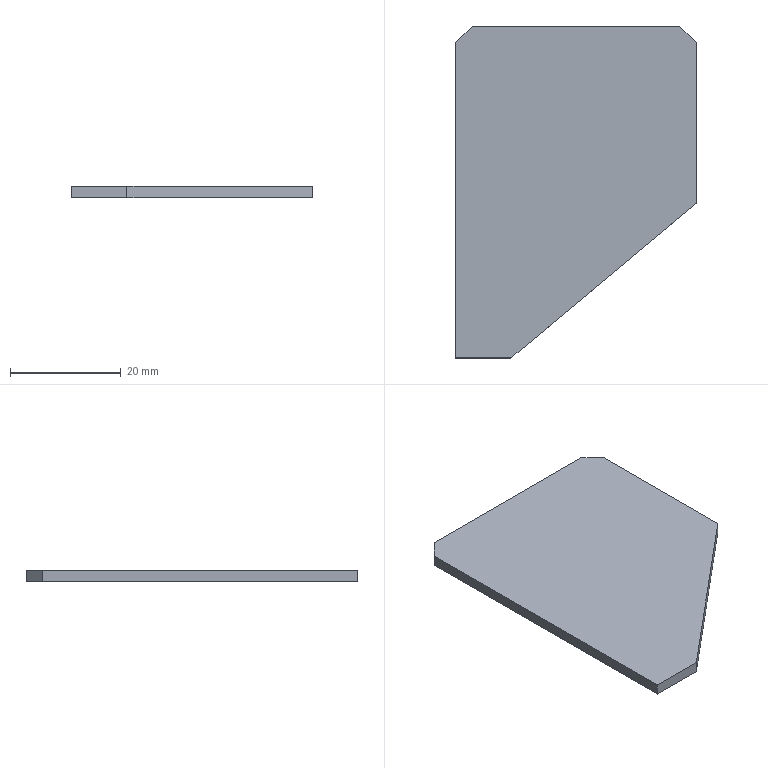Part | SolidWorks | features Chamfer 1, Extrusion 1 | 1 solid | 9 faces | box 43.5 x 60 x 2 mm | volume 4264 mm3 | plane 9
STEP:
#1=CARTESIAN_POINT('',(0.,-3.,2.));
#2=VERTEX_POINT('',#1);
#3=CARTESIAN_POINT('',(0.,-60.,2.));
#4=VERTEX_POINT('',#3);
#5=CARTESIAN_POINT('',(0.,-60.,2.));
#6=DIRECTION('',(0.,-1.,0.));
#7=VECTOR('',#6,1000.);
#8=LINE('',#5,#7);
#9=EDGE_CURVE('',#2,#4,#8,.T.);
#10=ORIENTED_EDGE('',*,*,#9,.F.);
#11=CARTESIAN_POINT('',(0.,-3.,0.));
#12=VERTEX_POINT('',#11);
#13=CARTESIAN_POINT('',(0.,-3.,2.));
#14=DIRECTION('',(0.,0.,-1.));
#15=VECTOR('',#14,1000.);
#16=LINE('',#13,#15);
#17=EDGE_CURVE('',#2,#12,#16,.T.);
#18=ORIENTED_EDGE('',*,*,#17,.T.);
#19=CARTESIAN_POINT('',(0.,-60.,0.));
#20=VERTEX_POINT('',#19);
#21=CARTESIAN_POINT('',(0.,-60.,0.));
#22=DIRECTION('',(0.,-1.,0.));
#23=VECTOR('',#22,1000.);
#24=LINE('',#21,#23);
#25=EDGE_CURVE('',#12,#20,#24,.T.);
#26=ORIENTED_EDGE('',*,*,#25,.T.);
#27=CARTESIAN_POINT('',(0.,-60.,2.));
#28=DIRECTION('',(0.,0.,-1.));
#29=VECTOR('',#28,1000.);
#30=LINE('',#27,#29);
#31=EDGE_CURVE('',#4,#20,#30,.T.);
#32=ORIENTED_EDGE('',*,*,#31,.F.);
#33=EDGE_LOOP('',(#10,#18,#26,#32));
#34=FACE_OUTER_BOUND('',#33,.T.);
#35=CARTESIAN_POINT('',(0.,-60.,2.));
#36=DIRECTION('',(1.,0.,0.));
#37=DIRECTION('',(0.,0.,-1.));
#38=AXIS2_PLACEMENT_3D('',#35,#36,#37);
#39=PLANE('',#38);
#40=ADVANCED_FACE('',(#34),#39,.F.);
#41=CARTESIAN_POINT('',(10.,-60.,0.));
#42=VERTEX_POINT('',#41);
#43=CARTESIAN_POINT('',(10.,-60.,0.));
#44=DIRECTION('',(1.,0.,0.));
#45=VECTOR('',#44,1000.);
#46=LINE('',#43,#45);
#47=EDGE_CURVE('',#20,#42,#46,.T.);
#48=ORIENTED_EDGE('',*,*,#47,.T.);
#49=CARTESIAN_POINT('',(10.,-60.,2.));
#50=VERTEX_POINT('',#49);
#51=CARTESIAN_POINT('',(10.,-60.,2.));
#52=DIRECTION('',(0.,0.,-1.));
#53=VECTOR('',#52,1000.);
#54=LINE('',#51,#53);
#55=EDGE_CURVE('',#50,#42,#54,.T.);
#56=ORIENTED_EDGE('',*,*,#55,.F.);
#57=CARTESIAN_POINT('',(10.,-60.,2.));
#58=DIRECTION('',(1.,0.,0.));
#59=VECTOR('',#58,1000.);
#60=LINE('',#57,#59);
#61=EDGE_CURVE('',#4,#50,#60,.T.);
#62=ORIENTED_EDGE('',*,*,#61,.F.);
#63=ORIENTED_EDGE('',*,*,#31,.T.);
#64=EDGE_LOOP('',(#48,#56,#62,#63));
#65=FACE_OUTER_BOUND('',#64,.T.);
#66=CARTESIAN_POINT('',(10.,-60.,2.));
#67=DIRECTION('',(0.,1.,0.));
#68=DIRECTION('',(0.,0.,1.));
#69=AXIS2_PLACEMENT_3D('',#66,#67,#68);
#70=PLANE('',#69);
#71=ADVANCED_FACE('',(#65),#70,.F.);
#72=CARTESIAN_POINT('',(43.5,-32.,0.));
#73=VERTEX_POINT('',#72);
#74=CARTESIAN_POINT('',(43.5,-32.,0.));
#75=DIRECTION('',(0.7673,0.6413,0.));
#76=VECTOR('',#75,1000.);
#77=LINE('',#74,#76);
#78=EDGE_CURVE('',#42,#73,#77,.T.);
#79=ORIENTED_EDGE('',*,*,#78,.T.);
#80=CARTESIAN_POINT('',(43.5,-32.,2.));
#81=VERTEX_POINT('',#80);
#82=CARTESIAN_POINT('',(43.5,-32.,2.));
#83=DIRECTION('',(0.,0.,-1.));
#84=VECTOR('',#83,1000.);
#85=LINE('',#82,#84);
#86=EDGE_CURVE('',#81,#73,#85,.T.);
#87=ORIENTED_EDGE('',*,*,#86,.F.);
#88=CARTESIAN_POINT('',(43.5,-32.,2.));
#89=DIRECTION('',(0.7673,0.6413,0.));
#90=VECTOR('',#89,1000.);
#91=LINE('',#88,#90);
#92=EDGE_CURVE('',#50,#81,#91,.T.);
#93=ORIENTED_EDGE('',*,*,#92,.F.);
#94=ORIENTED_EDGE('',*,*,#55,.T.);
#95=EDGE_LOOP('',(#79,#87,#93,#94));
#96=FACE_OUTER_BOUND('',#95,.T.);
#97=CARTESIAN_POINT('',(43.5,-32.,2.));
#98=DIRECTION('',(-0.6413,0.7673,0.));
#99=DIRECTION('',(-0.7673,-0.6413,0.));
#100=AXIS2_PLACEMENT_3D('',#97,#98,#99);
#101=PLANE('',#100);
#102=ADVANCED_FACE('',(#96),#101,.F.);
#103=CARTESIAN_POINT('',(43.5,-3.,0.));
#104=VERTEX_POINT('',#103);
#105=CARTESIAN_POINT('',(43.5,0.,0.));
#106=DIRECTION('',(0.,1.,0.));
#107=VECTOR('',#106,1000.);
#108=LINE('',#105,#107);
#109=EDGE_CURVE('',#73,#104,#108,.T.);
#110=ORIENTED_EDGE('',*,*,#109,.T.);
#111=CARTESIAN_POINT('',(43.5,-3.,2.));
#112=VERTEX_POINT('',#111);
#113=CARTESIAN_POINT('',(43.5,-3.,2.));
#114=DIRECTION('',(0.,0.,1.));
#115=VECTOR('',#114,1000.);
#116=LINE('',#113,#115);
#117=EDGE_CURVE('',#104,#112,#116,.T.);
#118=ORIENTED_EDGE('',*,*,#117,.T.);
#119=CARTESIAN_POINT('',(43.5,0.,2.));
#120=DIRECTION('',(0.,1.,0.));
#121=VECTOR('',#120,1000.);
#122=LINE('',#119,#121);
#123=EDGE_CURVE('',#81,#112,#122,.T.);
#124=ORIENTED_EDGE('',*,*,#123,.F.);
#125=ORIENTED_EDGE('',*,*,#86,.T.);
#126=EDGE_LOOP('',(#110,#118,#124,#125));
#127=FACE_OUTER_BOUND('',#126,.T.);
#128=CARTESIAN_POINT('',(43.5,0.,2.));
#129=DIRECTION('',(-1.,0.,0.));
#130=DIRECTION('',(0.,-1.,0.));
#131=AXIS2_PLACEMENT_3D('',#128,#129,#130);
#132=PLANE('',#131);
#133=ADVANCED_FACE('',(#127),#132,.F.);
#134=CARTESIAN_POINT('',(40.5,0.,2.));
#135=VERTEX_POINT('',#134);
#136=CARTESIAN_POINT('',(3.,0.,2.));
#137=VERTEX_POINT('',#136);
#138=CARTESIAN_POINT('',(0.,0.,2.));
#139=DIRECTION('',(-1.,0.,0.));
#140=VECTOR('',#139,1000.);
#141=LINE('',#138,#140);
#142=EDGE_CURVE('',#135,#137,#141,.T.);
#143=ORIENTED_EDGE('',*,*,#142,.F.);
#144=CARTESIAN_POINT('',(40.5,0.,0.));
#145=VERTEX_POINT('',#144);
#146=CARTESIAN_POINT('',(40.5,0.,2.));
#147=DIRECTION('',(0.,0.,-1.));
#148=VECTOR('',#147,1000.);
#149=LINE('',#146,#148);
#150=EDGE_CURVE('',#135,#145,#149,.T.);
#151=ORIENTED_EDGE('',*,*,#150,.T.);
#152=CARTESIAN_POINT('',(3.,0.,0.));
#153=VERTEX_POINT('',#152);
#154=CARTESIAN_POINT('',(0.,0.,0.));
#155=DIRECTION('',(-1.,0.,0.));
#156=VECTOR('',#155,1000.);
#157=LINE('',#154,#156);
#158=EDGE_CURVE('',#145,#153,#157,.T.);
#159=ORIENTED_EDGE('',*,*,#158,.T.);
#160=CARTESIAN_POINT('',(3.,0.,2.));
#161=DIRECTION('',(0.,0.,1.));
#162=VECTOR('',#161,1000.);
#163=LINE('',#160,#162);
#164=EDGE_CURVE('',#153,#137,#163,.T.);
#165=ORIENTED_EDGE('',*,*,#164,.T.);
#166=EDGE_LOOP('',(#143,#151,#159,#165));
#167=FACE_OUTER_BOUND('',#166,.T.);
#168=CARTESIAN_POINT('',(0.,0.,2.));
#169=DIRECTION('',(0.,-1.,0.));
#170=DIRECTION('',(0.,0.,-1.));
#171=AXIS2_PLACEMENT_3D('',#168,#169,#170);
#172=PLANE('',#171);
#173=ADVANCED_FACE('',(#167),#172,.F.);
#174=ORIENTED_EDGE('',*,*,#123,.T.);
#175=CARTESIAN_POINT('',(40.5,0.,2.));
#176=DIRECTION('',(-0.7071,0.7071,0.));
#177=VECTOR('',#176,1000.);
#178=LINE('',#175,#177);
#179=EDGE_CURVE('',#112,#135,#178,.T.);
#180=ORIENTED_EDGE('',*,*,#179,.T.);
#181=ORIENTED_EDGE('',*,*,#142,.T.);
#182=CARTESIAN_POINT('',(0.,-3.,2.));
#183=DIRECTION('',(-0.7071,-0.7071,0.));
#184=VECTOR('',#183,1000.);
#185=LINE('',#182,#184);
#186=EDGE_CURVE('',#137,#2,#185,.T.);
#187=ORIENTED_EDGE('',*,*,#186,.T.);
#188=ORIENTED_EDGE('',*,*,#9,.T.);
#189=ORIENTED_EDGE('',*,*,#61,.T.);
#190=ORIENTED_EDGE('',*,*,#92,.T.);
#191=EDGE_LOOP('',(#174,#180,#181,#187,#188,#189,#190));
#192=FACE_OUTER_BOUND('',#191,.T.);
#193=CARTESIAN_POINT('',(0.,0.,2.));
#194=DIRECTION('',(0.,0.,-1.));
#195=DIRECTION('',(-1.,0.,0.));
#196=AXIS2_PLACEMENT_3D('',#193,#194,#195);
#197=PLANE('',#196);
#198=ADVANCED_FACE('',(#192),#197,.F.);
#199=ORIENTED_EDGE('',*,*,#158,.F.);
#200=CARTESIAN_POINT('',(20.25,20.25,0.));
#201=DIRECTION('',(0.7071,-0.7071,0.));
#202=VECTOR('',#201,1000.);
#203=LINE('',#200,#202);
#204=EDGE_CURVE('',#145,#104,#203,.T.);
#205=ORIENTED_EDGE('',*,*,#204,.T.);
#206=ORIENTED_EDGE('',*,*,#109,.F.);
#207=ORIENTED_EDGE('',*,*,#78,.F.);
#208=ORIENTED_EDGE('',*,*,#47,.F.);
#209=ORIENTED_EDGE('',*,*,#25,.F.);
#210=CARTESIAN_POINT('',(1.5,-1.5,0.));
#211=DIRECTION('',(0.7071,0.7071,0.));
#212=VECTOR('',#211,1000.);
#213=LINE('',#210,#212);
#214=EDGE_CURVE('',#12,#153,#213,.T.);
#215=ORIENTED_EDGE('',*,*,#214,.T.);
#216=EDGE_LOOP('',(#199,#205,#206,#207,#208,#209,#215));
#217=FACE_OUTER_BOUND('',#216,.T.);
#218=CARTESIAN_POINT('',(0.,0.,0.));
#219=DIRECTION('',(0.,0.,-1.));
#220=DIRECTION('',(-1.,0.,0.));
#221=AXIS2_PLACEMENT_3D('',#218,#219,#220);
#222=PLANE('',#221);
#223=ADVANCED_FACE('',(#217),#222,.T.);
#224=ORIENTED_EDGE('',*,*,#179,.F.);
#225=ORIENTED_EDGE('',*,*,#117,.F.);
#226=ORIENTED_EDGE('',*,*,#204,.F.);
#227=ORIENTED_EDGE('',*,*,#150,.F.);
#228=EDGE_LOOP('',(#224,#225,#226,#227));
#229=FACE_OUTER_BOUND('',#228,.T.);
#230=CARTESIAN_POINT('',(40.5,0.,2.));
#231=DIRECTION('',(-0.7071,-0.7071,0.));
#232=DIRECTION('',(0.,0.,-1.));
#233=AXIS2_PLACEMENT_3D('',#230,#231,#232);
#234=PLANE('',#233);
#235=ADVANCED_FACE('',(#229),#234,.F.);
#236=ORIENTED_EDGE('',*,*,#186,.F.);
#237=ORIENTED_EDGE('',*,*,#164,.F.);
#238=ORIENTED_EDGE('',*,*,#214,.F.);
#239=ORIENTED_EDGE('',*,*,#17,.F.);
#240=EDGE_LOOP('',(#236,#237,#238,#239));
#241=FACE_OUTER_BOUND('',#240,.T.);
#242=CARTESIAN_POINT('',(0.,-3.,2.));
#243=DIRECTION('',(0.7071,-0.7071,0.));
#244=DIRECTION('',(0.,0.,-1.));
#245=AXIS2_PLACEMENT_3D('',#242,#243,#244);
#246=PLANE('',#245);
#247=ADVANCED_FACE('',(#241),#246,.F.);
#248=CLOSED_SHELL('',(#40,#71,#102,#133,#173,#198,#223,#235,#247));
#249=MANIFOLD_SOLID_BREP('',#248);
#250=CARTESIAN_POINT('',(0.,0.,0.));
#251=DIRECTION('',(0.,0.,1.));
#252=DIRECTION('',(1.,0.,0.));
#253=AXIS2_PLACEMENT_3D('',#250,#251,#252);
#254=(LENGTH_UNIT()NAMED_UNIT(*)SI_UNIT(.MILLI.,.METRE.));
#255=UNCERTAINTY_MEASURE_WITH_UNIT(LENGTH_MEASURE(0.00001),#254,'','');
#256=(NAMED_UNIT(*)PLANE_ANGLE_UNIT()SI_UNIT($,.RADIAN.));
#257=(NAMED_UNIT(*)SI_UNIT($,.STERADIAN.)SOLID_ANGLE_UNIT());
#258=(GEOMETRIC_REPRESENTATION_CONTEXT(3)GLOBAL_UNCERTAINTY_ASSIGNED_CONTEXT((#255))GLOBAL_UNIT_ASSIGNED_CONTEXT((#254,#256,#257))REPRESENTATION_CONTEXT('',''));
#259=ADVANCED_BREP_SHAPE_REPRESENTATION('',(#249,#253),#258);